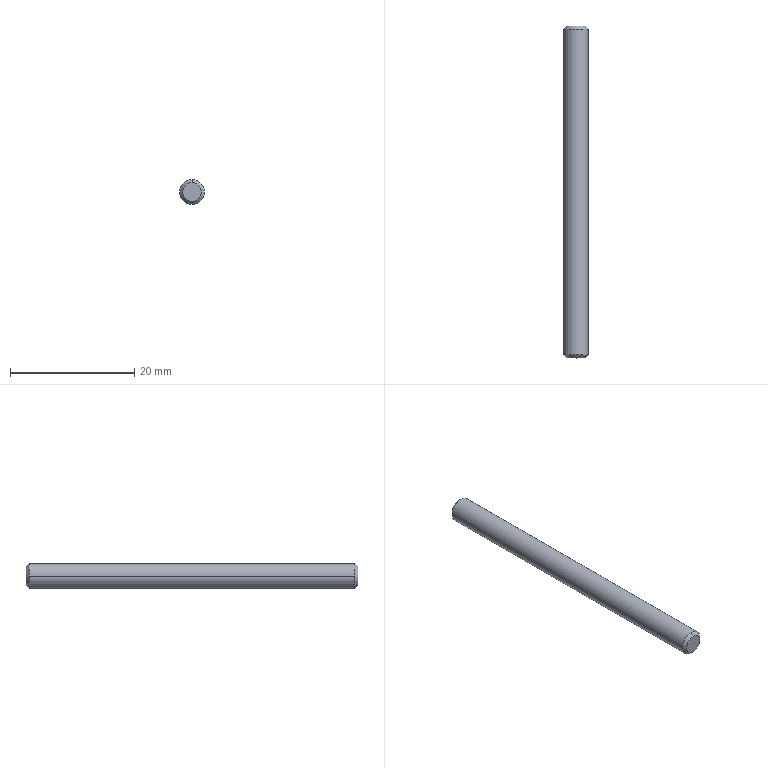Part | STEP file | 1 solid | 8 faces | box 4 x 53.4 x 4 mm | volume 668.164 mm3 | cone 4 | cylinder 2 | plane 2 | commonest cylinder face diameters 4 x2
STEP:
#1=CARTESIAN_POINT('',(0.,0.,0.));
#2=DIRECTION('',(0.,0.,1.));
#3=DIRECTION('',(1.,0.,0.));
#4=AXIS2_PLACEMENT_3D('',#1,#2,#3);
#5=CARTESIAN_POINT('',(0.,-26.7,-1.5));
#6=VERTEX_POINT('',#5);
#7=CARTESIAN_POINT('',(0.,-26.7,1.5));
#8=VERTEX_POINT('',#7);
#9=CARTESIAN_POINT('',(0.,-26.7,0.));
#10=DIRECTION('',(0.,-1.,0.));
#11=DIRECTION('',(0.,0.,1.));
#12=AXIS2_PLACEMENT_3D('',#9,#10,#11);
#13=CIRCLE('',#12,1.5);
#14=CARTESIAN_POINT('',(0.,-26.7,0.));
#15=DIRECTION('',(0.,1.,0.));
#16=DIRECTION('',(0.,0.,1.));
#17=AXIS2_PLACEMENT_3D('',#14,#15,#16);
#18=CONICAL_SURFACE('',#17,1.5,0.7854);
#19=CARTESIAN_POINT('',(6.283,0.));
#20=DIRECTION('',(-1.,0.));
#21=VECTOR('',#20,1.);
#22=LINE('',#19,#21);
#23=(GEOMETRIC_REPRESENTATION_CONTEXT(2)PARAMETRIC_REPRESENTATION_CONTEXT()REPRESENTATION_CONTEXT('',''));
#24=DEFINITIONAL_REPRESENTATION('',(#22),#23);
#25=PCURVE('',#18,#24);
#26=CARTESIAN_POINT('',(-1.518,-26.7,-1.518));
#27=DIRECTION('',(0.,1.,0.));
#28=DIRECTION('',(0.,0.,1.));
#29=AXIS2_PLACEMENT_3D('',#26,#27,#28);
#30=PLANE('',#29);
#31=CARTESIAN_POINT('',(3.018,1.518));
#32=CARTESIAN_POINT('',(3.018,-1.08));
#33=CARTESIAN_POINT('',(0.768,0.219));
#34=CARTESIAN_POINT('',(-1.482,1.518));
#35=CARTESIAN_POINT('',(0.768,2.817));
#36=CARTESIAN_POINT('',(3.018,4.116));
#37=CARTESIAN_POINT('',(3.018,1.518));
#38=(BOUNDED_CURVE()B_SPLINE_CURVE(2,(#31,#32,#33,#34,#35,#36,#37),.UNSPECIFIED.,.T.,.F.)B_SPLINE_CURVE_WITH_KNOTS((1,2,2,2,2,1),(-2.094,0.,2.094,4.189,6.283,8.378),.UNSPECIFIED.)CURVE()GEOMETRIC_REPRESENTATION_ITEM()RATIONAL_B_SPLINE_CURVE((1.,0.5,1.,0.5,1.,0.5,1.))REPRESENTATION_ITEM(''));
#39=(GEOMETRIC_REPRESENTATION_CONTEXT(2)PARAMETRIC_REPRESENTATION_CONTEXT()REPRESENTATION_CONTEXT('',''));
#40=DEFINITIONAL_REPRESENTATION('',(#38),#39);
#41=PCURVE('',#30,#40);
#42=SURFACE_CURVE('',#13,(#25,#41),.PCURVE_S1.);
#43=EDGE_CURVE('',#6,#8,#42,.T.);
#44=ORIENTED_EDGE('',*,*,#43,.F.);
#45=CARTESIAN_POINT('',(0.,-26.2,-2.));
#46=VERTEX_POINT('',#45);
#47=CARTESIAN_POINT('',(0.,-26.7,-1.5));
#48=DIRECTION('',(0.,0.7071,-0.7071));
#49=VECTOR('',#48,1.);
#50=LINE('',#47,#49);
#51=CARTESIAN_POINT('',(3.142,0.));
#52=DIRECTION('',(0.,1.));
#53=VECTOR('',#52,1.);
#54=LINE('',#51,#53);
#55=(GEOMETRIC_REPRESENTATION_CONTEXT(2)PARAMETRIC_REPRESENTATION_CONTEXT()REPRESENTATION_CONTEXT('',''));
#56=DEFINITIONAL_REPRESENTATION('',(#54),#55);
#57=PCURVE('',#18,#56);
#58=CARTESIAN_POINT('',(0.,-26.7,0.));
#59=DIRECTION('',(0.,1.,0.));
#60=DIRECTION('',(0.,0.,1.));
#61=AXIS2_PLACEMENT_3D('',#58,#59,#60);
#62=CONICAL_SURFACE('',#61,1.5,0.7854);
#63=CARTESIAN_POINT('',(3.142,0.));
#64=DIRECTION('',(0.,1.));
#65=VECTOR('',#64,1.);
#66=LINE('',#63,#65);
#67=(GEOMETRIC_REPRESENTATION_CONTEXT(2)PARAMETRIC_REPRESENTATION_CONTEXT()REPRESENTATION_CONTEXT('',''));
#68=DEFINITIONAL_REPRESENTATION('',(#66),#67);
#69=PCURVE('',#62,#68);
#70=SURFACE_CURVE('',#50,(#57,#69),.PCURVE_S1.);
#71=EDGE_CURVE('',#6,#46,#70,.T.);
#72=ORIENTED_EDGE('',*,*,#71,.T.);
#73=CARTESIAN_POINT('',(2.,-26.2,0.));
#74=VERTEX_POINT('',#73);
#75=CARTESIAN_POINT('',(0.,-26.2,0.));
#76=DIRECTION('',(0.,1.,0.));
#77=DIRECTION('',(0.,0.,1.));
#78=AXIS2_PLACEMENT_3D('',#75,#76,#77);
#79=CIRCLE('',#78,2.);
#80=CARTESIAN_POINT('',(0.,0.5));
#81=DIRECTION('',(1.,0.));
#82=VECTOR('',#81,1.);
#83=LINE('',#80,#82);
#84=(GEOMETRIC_REPRESENTATION_CONTEXT(2)PARAMETRIC_REPRESENTATION_CONTEXT()REPRESENTATION_CONTEXT('',''));
#85=DEFINITIONAL_REPRESENTATION('',(#83),#84);
#86=PCURVE('',#18,#85);
#87=CARTESIAN_POINT('',(0.,-26.2,0.));
#88=DIRECTION('',(0.,1.,0.));
#89=DIRECTION('',(-1.,0.,0.));
#90=AXIS2_PLACEMENT_3D('',#87,#88,#89);
#91=CYLINDRICAL_SURFACE('',#90,2.);
#92=CARTESIAN_POINT('',(1.571,0.));
#93=DIRECTION('',(1.,0.));
#94=VECTOR('',#93,1.);
#95=LINE('',#92,#94);
#96=(GEOMETRIC_REPRESENTATION_CONTEXT(2)PARAMETRIC_REPRESENTATION_CONTEXT()REPRESENTATION_CONTEXT('',''));
#97=DEFINITIONAL_REPRESENTATION('',(#95),#96);
#98=PCURVE('',#91,#97);
#99=SURFACE_CURVE('',#79,(#86,#98),.PCURVE_S1.);
#100=EDGE_CURVE('',#74,#46,#99,.T.);
#101=ORIENTED_EDGE('',*,*,#100,.F.);
#102=CARTESIAN_POINT('',(0.,-26.2,2.));
#103=VERTEX_POINT('',#102);
#104=CARTESIAN_POINT('',(0.,-26.2,0.));
#105=DIRECTION('',(0.,1.,0.));
#106=DIRECTION('',(0.,0.,1.));
#107=AXIS2_PLACEMENT_3D('',#104,#105,#106);
#108=CIRCLE('',#107,2.);
#109=CARTESIAN_POINT('',(0.,0.5));
#110=DIRECTION('',(1.,0.));
#111=VECTOR('',#110,1.);
#112=LINE('',#109,#111);
#113=(GEOMETRIC_REPRESENTATION_CONTEXT(2)PARAMETRIC_REPRESENTATION_CONTEXT()REPRESENTATION_CONTEXT('',''));
#114=DEFINITIONAL_REPRESENTATION('',(#112),#113);
#115=PCURVE('',#18,#114);
#116=CARTESIAN_POINT('',(0.,-26.2,0.));
#117=DIRECTION('',(0.,1.,0.));
#118=DIRECTION('',(-1.,0.,0.));
#119=AXIS2_PLACEMENT_3D('',#116,#117,#118);
#120=CYLINDRICAL_SURFACE('',#119,2.);
#121=CARTESIAN_POINT('',(1.571,0.));
#122=DIRECTION('',(1.,0.));
#123=VECTOR('',#122,1.);
#124=LINE('',#121,#123);
#125=(GEOMETRIC_REPRESENTATION_CONTEXT(2)PARAMETRIC_REPRESENTATION_CONTEXT()REPRESENTATION_CONTEXT('',''));
#126=DEFINITIONAL_REPRESENTATION('',(#124),#125);
#127=PCURVE('',#120,#126);
#128=SURFACE_CURVE('',#108,(#115,#127),.PCURVE_S1.);
#129=EDGE_CURVE('',#103,#74,#128,.T.);
#130=ORIENTED_EDGE('',*,*,#129,.F.);
#131=CARTESIAN_POINT('',(0.,-26.7,1.5));
#132=DIRECTION('',(0.,0.7071,0.7071));
#133=VECTOR('',#132,1.);
#134=LINE('',#131,#133);
#135=CARTESIAN_POINT('',(0.,0.));
#136=DIRECTION('',(0.,1.));
#137=VECTOR('',#136,1.);
#138=LINE('',#135,#137);
#139=(GEOMETRIC_REPRESENTATION_CONTEXT(2)PARAMETRIC_REPRESENTATION_CONTEXT()REPRESENTATION_CONTEXT('',''));
#140=DEFINITIONAL_REPRESENTATION('',(#138),#139);
#141=PCURVE('',#18,#140);
#142=CARTESIAN_POINT('',(6.283,0.));
#143=DIRECTION('',(0.,1.));
#144=VECTOR('',#143,1.);
#145=LINE('',#142,#144);
#146=(GEOMETRIC_REPRESENTATION_CONTEXT(2)PARAMETRIC_REPRESENTATION_CONTEXT()REPRESENTATION_CONTEXT('',''));
#147=DEFINITIONAL_REPRESENTATION('',(#145),#146);
#148=PCURVE('',#62,#147);
#149=SURFACE_CURVE('',#134,(#141,#148),.PCURVE_S1.);
#150=EDGE_CURVE('',#8,#103,#149,.T.);
#151=ORIENTED_EDGE('',*,*,#150,.F.);
#152=EDGE_LOOP('',(#44,#72,#101,#130,#151));
#153=FACE_BOUND('',#152,.T.);
#154=ADVANCED_FACE('',(#153),#18,.T.);
#155=CARTESIAN_POINT('',(-2.,-26.2,0.));
#156=VERTEX_POINT('',#155);
#157=CARTESIAN_POINT('',(0.,-26.2,0.));
#158=DIRECTION('',(0.,1.,0.));
#159=DIRECTION('',(0.,0.,1.));
#160=AXIS2_PLACEMENT_3D('',#157,#158,#159);
#161=CIRCLE('',#160,2.);
#162=CARTESIAN_POINT('',(-4.712,0.));
#163=DIRECTION('',(1.,0.));
#164=VECTOR('',#163,1.);
#165=LINE('',#162,#164);
#166=(GEOMETRIC_REPRESENTATION_CONTEXT(2)PARAMETRIC_REPRESENTATION_CONTEXT()REPRESENTATION_CONTEXT('',''));
#167=DEFINITIONAL_REPRESENTATION('',(#165),#166);
#168=PCURVE('',#120,#167);
#169=CARTESIAN_POINT('',(0.,0.5));
#170=DIRECTION('',(1.,0.));
#171=VECTOR('',#170,1.);
#172=LINE('',#169,#171);
#173=(GEOMETRIC_REPRESENTATION_CONTEXT(2)PARAMETRIC_REPRESENTATION_CONTEXT()REPRESENTATION_CONTEXT('',''));
#174=DEFINITIONAL_REPRESENTATION('',(#172),#173);
#175=PCURVE('',#62,#174);
#176=SURFACE_CURVE('',#161,(#168,#175),.PCURVE_S1.);
#177=EDGE_CURVE('',#156,#103,#176,.T.);
#178=ORIENTED_EDGE('',*,*,#177,.T.);
#179=ORIENTED_EDGE('',*,*,#129,.T.);
#180=CARTESIAN_POINT('',(2.,26.2,0.));
#181=VERTEX_POINT('',#180);
#182=CARTESIAN_POINT('',(2.,-26.2,0.));
#183=DIRECTION('',(0.,1.,0.));
#184=VECTOR('',#183,1.);
#185=LINE('',#182,#184);
#186=CARTESIAN_POINT('',(3.142,0.));
#187=DIRECTION('',(0.,1.));
#188=VECTOR('',#187,1.);
#189=LINE('',#186,#188);
#190=(GEOMETRIC_REPRESENTATION_CONTEXT(2)PARAMETRIC_REPRESENTATION_CONTEXT()REPRESENTATION_CONTEXT('',''));
#191=DEFINITIONAL_REPRESENTATION('',(#189),#190);
#192=PCURVE('',#120,#191);
#193=CARTESIAN_POINT('',(3.142,0.));
#194=DIRECTION('',(0.,1.));
#195=VECTOR('',#194,1.);
#196=LINE('',#193,#195);
#197=(GEOMETRIC_REPRESENTATION_CONTEXT(2)PARAMETRIC_REPRESENTATION_CONTEXT()REPRESENTATION_CONTEXT('',''));
#198=DEFINITIONAL_REPRESENTATION('',(#196),#197);
#199=PCURVE('',#91,#198);
#200=SURFACE_CURVE('',#185,(#192,#199),.PCURVE_S1.);
#201=EDGE_CURVE('',#74,#181,#200,.T.);
#202=ORIENTED_EDGE('',*,*,#201,.T.);
#203=CARTESIAN_POINT('',(0.,26.2,2.));
#204=VERTEX_POINT('',#203);
#205=CARTESIAN_POINT('',(0.,26.2,0.));
#206=DIRECTION('',(0.,1.,0.));
#207=DIRECTION('',(0.,0.,1.));
#208=AXIS2_PLACEMENT_3D('',#205,#206,#207);
#209=CIRCLE('',#208,2.);
#210=CARTESIAN_POINT('',(1.571,52.4));
#211=DIRECTION('',(1.,0.));
#212=VECTOR('',#211,1.);
#213=LINE('',#210,#212);
#214=(GEOMETRIC_REPRESENTATION_CONTEXT(2)PARAMETRIC_REPRESENTATION_CONTEXT()REPRESENTATION_CONTEXT('',''));
#215=DEFINITIONAL_REPRESENTATION('',(#213),#214);
#216=PCURVE('',#120,#215);
#217=CARTESIAN_POINT('',(0.,26.7,0.));
#218=DIRECTION('',(0.,-1.,0.));
#219=DIRECTION('',(0.,0.,-1.));
#220=AXIS2_PLACEMENT_3D('',#217,#218,#219);
#221=CONICAL_SURFACE('',#220,1.5,0.7854);
#222=CARTESIAN_POINT('',(3.142,0.5));
#223=DIRECTION('',(-1.,0.));
#224=VECTOR('',#223,1.);
#225=LINE('',#222,#224);
#226=(GEOMETRIC_REPRESENTATION_CONTEXT(2)PARAMETRIC_REPRESENTATION_CONTEXT()REPRESENTATION_CONTEXT('',''));
#227=DEFINITIONAL_REPRESENTATION('',(#225),#226);
#228=PCURVE('',#221,#227);
#229=SURFACE_CURVE('',#209,(#216,#228),.PCURVE_S1.);
#230=EDGE_CURVE('',#204,#181,#229,.T.);
#231=ORIENTED_EDGE('',*,*,#230,.F.);
#232=CARTESIAN_POINT('',(-2.,26.2,0.));
#233=VERTEX_POINT('',#232);
#234=CARTESIAN_POINT('',(0.,26.2,0.));
#235=DIRECTION('',(0.,1.,0.));
#236=DIRECTION('',(0.,0.,1.));
#237=AXIS2_PLACEMENT_3D('',#234,#235,#236);
#238=CIRCLE('',#237,2.);
#239=CARTESIAN_POINT('',(-4.712,52.4));
#240=DIRECTION('',(1.,0.));
#241=VECTOR('',#240,1.);
#242=LINE('',#239,#241);
#243=(GEOMETRIC_REPRESENTATION_CONTEXT(2)PARAMETRIC_REPRESENTATION_CONTEXT()REPRESENTATION_CONTEXT('',''));
#244=DEFINITIONAL_REPRESENTATION('',(#242),#243);
#245=PCURVE('',#120,#244);
#246=CARTESIAN_POINT('',(0.,26.7,0.));
#247=DIRECTION('',(0.,-1.,0.));
#248=DIRECTION('',(0.,0.,-1.));
#249=AXIS2_PLACEMENT_3D('',#246,#247,#248);
#250=CONICAL_SURFACE('',#249,1.5,0.7854);
#251=CARTESIAN_POINT('',(9.425,0.5));
#252=DIRECTION('',(-1.,0.));
#253=VECTOR('',#252,1.);
#254=LINE('',#251,#253);
#255=(GEOMETRIC_REPRESENTATION_CONTEXT(2)PARAMETRIC_REPRESENTATION_CONTEXT()REPRESENTATION_CONTEXT('',''));
#256=DEFINITIONAL_REPRESENTATION('',(#254),#255);
#257=PCURVE('',#250,#256);
#258=SURFACE_CURVE('',#238,(#245,#257),.PCURVE_S1.);
#259=EDGE_CURVE('',#233,#204,#258,.T.);
#260=ORIENTED_EDGE('',*,*,#259,.F.);
#261=CARTESIAN_POINT('',(-2.,-26.2,0.));
#262=DIRECTION('',(0.,1.,0.));
#263=VECTOR('',#262,1.);
#264=LINE('',#261,#263);
#265=CARTESIAN_POINT('',(0.,0.));
#266=DIRECTION('',(0.,1.));
#267=VECTOR('',#266,1.);
#268=LINE('',#265,#267);
#269=(GEOMETRIC_REPRESENTATION_CONTEXT(2)PARAMETRIC_REPRESENTATION_CONTEXT()REPRESENTATION_CONTEXT('',''));
#270=DEFINITIONAL_REPRESENTATION('',(#268),#269);
#271=PCURVE('',#120,#270);
#272=CARTESIAN_POINT('',(6.283,0.));
#273=DIRECTION('',(0.,1.));
#274=VECTOR('',#273,1.);
#275=LINE('',#272,#274);
#276=(GEOMETRIC_REPRESENTATION_CONTEXT(2)PARAMETRIC_REPRESENTATION_CONTEXT()REPRESENTATION_CONTEXT('',''));
#277=DEFINITIONAL_REPRESENTATION('',(#275),#276);
#278=PCURVE('',#91,#277);
#279=SURFACE_CURVE('',#264,(#271,#278),.PCURVE_S1.);
#280=EDGE_CURVE('',#156,#233,#279,.T.);
#281=ORIENTED_EDGE('',*,*,#280,.F.);
#282=EDGE_LOOP('',(#178,#179,#202,#231,#260,#281));
#283=FACE_BOUND('',#282,.T.);
#284=ADVANCED_FACE('',(#283),#120,.T.);
#285=CARTESIAN_POINT('',(0.,26.7,1.5));
#286=VERTEX_POINT('',#285);
#287=CARTESIAN_POINT('',(0.,26.7,-1.5));
#288=VERTEX_POINT('',#287);
#289=CARTESIAN_POINT('',(0.,26.7,0.));
#290=DIRECTION('',(0.,1.,0.));
#291=DIRECTION('',(0.,0.,-1.));
#292=AXIS2_PLACEMENT_3D('',#289,#290,#291);
#293=CIRCLE('',#292,1.5);
#294=CARTESIAN_POINT('',(6.283,0.));
#295=DIRECTION('',(-1.,0.));
#296=VECTOR('',#295,1.);
#297=LINE('',#294,#296);
#298=(GEOMETRIC_REPRESENTATION_CONTEXT(2)PARAMETRIC_REPRESENTATION_CONTEXT()REPRESENTATION_CONTEXT('',''));
#299=DEFINITIONAL_REPRESENTATION('',(#297),#298);
#300=PCURVE('',#221,#299);
#301=CARTESIAN_POINT('',(-1.518,26.7,1.518));
#302=DIRECTION('',(0.,-1.,0.));
#303=DIRECTION('',(0.,0.,-1.));
#304=AXIS2_PLACEMENT_3D('',#301,#302,#303);
#305=PLANE('',#304);
#306=CARTESIAN_POINT('',(3.018,1.518));
#307=CARTESIAN_POINT('',(3.018,-1.08));
#308=CARTESIAN_POINT('',(0.768,0.219));
#309=CARTESIAN_POINT('',(-1.482,1.518));
#310=CARTESIAN_POINT('',(0.768,2.817));
#311=CARTESIAN_POINT('',(3.018,4.116));
#312=CARTESIAN_POINT('',(3.018,1.518));
#313=(BOUNDED_CURVE()B_SPLINE_CURVE(2,(#306,#307,#308,#309,#310,#311,#312),.UNSPECIFIED.,.T.,.F.)B_SPLINE_CURVE_WITH_KNOTS((1,2,2,2,2,1),(-2.094,0.,2.094,4.189,6.283,8.378),.UNSPECIFIED.)CURVE()GEOMETRIC_REPRESENTATION_ITEM()RATIONAL_B_SPLINE_CURVE((1.,0.5,1.,0.5,1.,0.5,1.))REPRESENTATION_ITEM(''));
#314=(GEOMETRIC_REPRESENTATION_CONTEXT(2)PARAMETRIC_REPRESENTATION_CONTEXT()REPRESENTATION_CONTEXT('',''));
#315=DEFINITIONAL_REPRESENTATION('',(#313),#314);
#316=PCURVE('',#305,#315);
#317=SURFACE_CURVE('',#293,(#300,#316),.PCURVE_S1.);
#318=EDGE_CURVE('',#286,#288,#317,.T.);
#319=ORIENTED_EDGE('',*,*,#318,.F.);
#320=CARTESIAN_POINT('',(0.,26.7,1.5));
#321=DIRECTION('',(0.,-0.7071,0.7071));
#322=VECTOR('',#321,1.);
#323=LINE('',#320,#322);
#324=CARTESIAN_POINT('',(3.142,0.));
#325=DIRECTION('',(0.,1.));
#326=VECTOR('',#325,1.);
#327=LINE('',#324,#326);
#328=(GEOMETRIC_REPRESENTATION_CONTEXT(2)PARAMETRIC_REPRESENTATION_CONTEXT()REPRESENTATION_CONTEXT('',''));
#329=DEFINITIONAL_REPRESENTATION('',(#327),#328);
#330=PCURVE('',#221,#329);
#331=CARTESIAN_POINT('',(3.142,0.));
#332=DIRECTION('',(0.,1.));
#333=VECTOR('',#332,1.);
#334=LINE('',#331,#333);
#335=(GEOMETRIC_REPRESENTATION_CONTEXT(2)PARAMETRIC_REPRESENTATION_CONTEXT()REPRESENTATION_CONTEXT('',''));
#336=DEFINITIONAL_REPRESENTATION('',(#334),#335);
#337=PCURVE('',#250,#336);
#338=SURFACE_CURVE('',#323,(#330,#337),.PCURVE_S1.);
#339=EDGE_CURVE('',#286,#204,#338,.T.);
#340=ORIENTED_EDGE('',*,*,#339,.T.);
#341=ORIENTED_EDGE('',*,*,#230,.T.);
#342=CARTESIAN_POINT('',(0.,26.2,-2.));
#343=VERTEX_POINT('',#342);
#344=CARTESIAN_POINT('',(0.,26.2,0.));
#345=DIRECTION('',(0.,1.,0.));
#346=DIRECTION('',(0.,0.,1.));
#347=AXIS2_PLACEMENT_3D('',#344,#345,#346);
#348=CIRCLE('',#347,2.);
#349=CARTESIAN_POINT('',(3.142,0.5));
#350=DIRECTION('',(-1.,0.));
#351=VECTOR('',#350,1.);
#352=LINE('',#349,#351);
#353=(GEOMETRIC_REPRESENTATION_CONTEXT(2)PARAMETRIC_REPRESENTATION_CONTEXT()REPRESENTATION_CONTEXT('',''));
#354=DEFINITIONAL_REPRESENTATION('',(#352),#353);
#355=PCURVE('',#221,#354);
#356=CARTESIAN_POINT('',(1.571,52.4));
#357=DIRECTION('',(1.,0.));
#358=VECTOR('',#357,1.);
#359=LINE('',#356,#358);
#360=(GEOMETRIC_REPRESENTATION_CONTEXT(2)PARAMETRIC_REPRESENTATION_CONTEXT()REPRESENTATION_CONTEXT('',''));
#361=DEFINITIONAL_REPRESENTATION('',(#359),#360);
#362=PCURVE('',#91,#361);
#363=SURFACE_CURVE('',#348,(#355,#362),.PCURVE_S1.);
#364=EDGE_CURVE('',#181,#343,#363,.T.);
#365=ORIENTED_EDGE('',*,*,#364,.T.);
#366=CARTESIAN_POINT('',(0.,26.7,-1.5));
#367=DIRECTION('',(0.,-0.7071,-0.7071));
#368=VECTOR('',#367,1.);
#369=LINE('',#366,#368);
#370=CARTESIAN_POINT('',(0.,0.));
#371=DIRECTION('',(0.,1.));
#372=VECTOR('',#371,1.);
#373=LINE('',#370,#372);
#374=(GEOMETRIC_REPRESENTATION_CONTEXT(2)PARAMETRIC_REPRESENTATION_CONTEXT()REPRESENTATION_CONTEXT('',''));
#375=DEFINITIONAL_REPRESENTATION('',(#373),#374);
#376=PCURVE('',#221,#375);
#377=CARTESIAN_POINT('',(6.283,0.));
#378=DIRECTION('',(0.,1.));
#379=VECTOR('',#378,1.);
#380=LINE('',#377,#379);
#381=(GEOMETRIC_REPRESENTATION_CONTEXT(2)PARAMETRIC_REPRESENTATION_CONTEXT()REPRESENTATION_CONTEXT('',''));
#382=DEFINITIONAL_REPRESENTATION('',(#380),#381);
#383=PCURVE('',#250,#382);
#384=SURFACE_CURVE('',#369,(#376,#383),.PCURVE_S1.);
#385=EDGE_CURVE('',#288,#343,#384,.T.);
#386=ORIENTED_EDGE('',*,*,#385,.F.);
#387=EDGE_LOOP('',(#319,#340,#341,#365,#386));
#388=FACE_BOUND('',#387,.T.);
#389=ADVANCED_FACE('',(#388),#221,.T.);
#390=ORIENTED_EDGE('',*,*,#71,.F.);
#391=CARTESIAN_POINT('',(0.,-26.7,0.));
#392=DIRECTION('',(0.,-1.,0.));
#393=DIRECTION('',(0.,0.,1.));
#394=AXIS2_PLACEMENT_3D('',#391,#392,#393);
#395=CIRCLE('',#394,1.5);
#396=CARTESIAN_POINT('',(6.283,0.));
#397=DIRECTION('',(-1.,0.));
#398=VECTOR('',#397,1.);
#399=LINE('',#396,#398);
#400=(GEOMETRIC_REPRESENTATION_CONTEXT(2)PARAMETRIC_REPRESENTATION_CONTEXT()REPRESENTATION_CONTEXT('',''));
#401=DEFINITIONAL_REPRESENTATION('',(#399),#400);
#402=PCURVE('',#62,#401);
#403=CARTESIAN_POINT('',(3.018,1.518));
#404=CARTESIAN_POINT('',(3.018,-1.08));
#405=CARTESIAN_POINT('',(0.768,0.219));
#406=CARTESIAN_POINT('',(-1.482,1.518));
#407=CARTESIAN_POINT('',(0.768,2.817));
#408=CARTESIAN_POINT('',(3.018,4.116));
#409=CARTESIAN_POINT('',(3.018,1.518));
#410=(BOUNDED_CURVE()B_SPLINE_CURVE(2,(#403,#404,#405,#406,#407,#408,#409),.UNSPECIFIED.,.T.,.F.)B_SPLINE_CURVE_WITH_KNOTS((1,2,2,2,2,1),(-2.094,0.,2.094,4.189,6.283,8.378),.UNSPECIFIED.)CURVE()GEOMETRIC_REPRESENTATION_ITEM()RATIONAL_B_SPLINE_CURVE((1.,0.5,1.,0.5,1.,0.5,1.))REPRESENTATION_ITEM(''));
#411=(GEOMETRIC_REPRESENTATION_CONTEXT(2)PARAMETRIC_REPRESENTATION_CONTEXT()REPRESENTATION_CONTEXT('',''));
#412=DEFINITIONAL_REPRESENTATION('',(#410),#411);
#413=PCURVE('',#30,#412);
#414=SURFACE_CURVE('',#395,(#402,#413),.PCURVE_S1.);
#415=EDGE_CURVE('',#8,#6,#414,.T.);
#416=ORIENTED_EDGE('',*,*,#415,.F.);
#417=ORIENTED_EDGE('',*,*,#150,.T.);
#418=ORIENTED_EDGE('',*,*,#177,.F.);
#419=CARTESIAN_POINT('',(0.,-26.2,0.));
#420=DIRECTION('',(0.,1.,0.));
#421=DIRECTION('',(0.,0.,1.));
#422=AXIS2_PLACEMENT_3D('',#419,#420,#421);
#423=CIRCLE('',#422,2.);
#424=CARTESIAN_POINT('',(0.,0.5));
#425=DIRECTION('',(1.,0.));
#426=VECTOR('',#425,1.);
#427=LINE('',#424,#426);
#428=(GEOMETRIC_REPRESENTATION_CONTEXT(2)PARAMETRIC_REPRESENTATION_CONTEXT()REPRESENTATION_CONTEXT('',''));
#429=DEFINITIONAL_REPRESENTATION('',(#427),#428);
#430=PCURVE('',#62,#429);
#431=CARTESIAN_POINT('',(1.571,0.));
#432=DIRECTION('',(1.,0.));
#433=VECTOR('',#432,1.);
#434=LINE('',#431,#433);
#435=(GEOMETRIC_REPRESENTATION_CONTEXT(2)PARAMETRIC_REPRESENTATION_CONTEXT()REPRESENTATION_CONTEXT('',''));
#436=DEFINITIONAL_REPRESENTATION('',(#434),#435);
#437=PCURVE('',#91,#436);
#438=SURFACE_CURVE('',#423,(#430,#437),.PCURVE_S1.);
#439=EDGE_CURVE('',#46,#156,#438,.T.);
#440=ORIENTED_EDGE('',*,*,#439,.F.);
#441=EDGE_LOOP('',(#390,#416,#417,#418,#440));
#442=FACE_BOUND('',#441,.T.);
#443=ADVANCED_FACE('',(#442),#62,.T.);
#444=ORIENTED_EDGE('',*,*,#415,.T.);
#445=ORIENTED_EDGE('',*,*,#43,.T.);
#446=EDGE_LOOP('',(#444,#445));
#447=FACE_BOUND('',#446,.T.);
#448=ADVANCED_FACE('',(#447),#30,.F.);
#449=ORIENTED_EDGE('',*,*,#201,.F.);
#450=ORIENTED_EDGE('',*,*,#100,.T.);
#451=ORIENTED_EDGE('',*,*,#439,.T.);
#452=ORIENTED_EDGE('',*,*,#280,.T.);
#453=CARTESIAN_POINT('',(0.,26.2,0.));
#454=DIRECTION('',(0.,1.,0.));
#455=DIRECTION('',(0.,0.,1.));
#456=AXIS2_PLACEMENT_3D('',#453,#454,#455);
#457=CIRCLE('',#456,2.);
#458=CARTESIAN_POINT('',(1.571,52.4));
#459=DIRECTION('',(1.,0.));
#460=VECTOR('',#459,1.);
#461=LINE('',#458,#460);
#462=(GEOMETRIC_REPRESENTATION_CONTEXT(2)PARAMETRIC_REPRESENTATION_CONTEXT()REPRESENTATION_CONTEXT('',''));
#463=DEFINITIONAL_REPRESENTATION('',(#461),#462);
#464=PCURVE('',#91,#463);
#465=CARTESIAN_POINT('',(9.425,0.5));
#466=DIRECTION('',(-1.,0.));
#467=VECTOR('',#466,1.);
#468=LINE('',#465,#467);
#469=(GEOMETRIC_REPRESENTATION_CONTEXT(2)PARAMETRIC_REPRESENTATION_CONTEXT()REPRESENTATION_CONTEXT('',''));
#470=DEFINITIONAL_REPRESENTATION('',(#468),#469);
#471=PCURVE('',#250,#470);
#472=SURFACE_CURVE('',#457,(#464,#471),.PCURVE_S1.);
#473=EDGE_CURVE('',#343,#233,#472,.T.);
#474=ORIENTED_EDGE('',*,*,#473,.F.);
#475=ORIENTED_EDGE('',*,*,#364,.F.);
#476=EDGE_LOOP('',(#449,#450,#451,#452,#474,#475));
#477=FACE_BOUND('',#476,.T.);
#478=ADVANCED_FACE('',(#477),#91,.T.);
#479=ORIENTED_EDGE('',*,*,#339,.F.);
#480=CARTESIAN_POINT('',(0.,26.7,0.));
#481=DIRECTION('',(0.,1.,0.));
#482=DIRECTION('',(0.,0.,-1.));
#483=AXIS2_PLACEMENT_3D('',#480,#481,#482);
#484=CIRCLE('',#483,1.5);
#485=CARTESIAN_POINT('',(6.283,0.));
#486=DIRECTION('',(-1.,0.));
#487=VECTOR('',#486,1.);
#488=LINE('',#485,#487);
#489=(GEOMETRIC_REPRESENTATION_CONTEXT(2)PARAMETRIC_REPRESENTATION_CONTEXT()REPRESENTATION_CONTEXT('',''));
#490=DEFINITIONAL_REPRESENTATION('',(#488),#489);
#491=PCURVE('',#250,#490);
#492=CARTESIAN_POINT('',(3.018,1.518));
#493=CARTESIAN_POINT('',(3.018,-1.08));
#494=CARTESIAN_POINT('',(0.768,0.219));
#495=CARTESIAN_POINT('',(-1.482,1.518));
#496=CARTESIAN_POINT('',(0.768,2.817));
#497=CARTESIAN_POINT('',(3.018,4.116));
#498=CARTESIAN_POINT('',(3.018,1.518));
#499=(BOUNDED_CURVE()B_SPLINE_CURVE(2,(#492,#493,#494,#495,#496,#497,#498),.UNSPECIFIED.,.T.,.F.)B_SPLINE_CURVE_WITH_KNOTS((1,2,2,2,2,1),(-2.094,0.,2.094,4.189,6.283,8.378),.UNSPECIFIED.)CURVE()GEOMETRIC_REPRESENTATION_ITEM()RATIONAL_B_SPLINE_CURVE((1.,0.5,1.,0.5,1.,0.5,1.))REPRESENTATION_ITEM(''));
#500=(GEOMETRIC_REPRESENTATION_CONTEXT(2)PARAMETRIC_REPRESENTATION_CONTEXT()REPRESENTATION_CONTEXT('',''));
#501=DEFINITIONAL_REPRESENTATION('',(#499),#500);
#502=PCURVE('',#305,#501);
#503=SURFACE_CURVE('',#484,(#491,#502),.PCURVE_S1.);
#504=EDGE_CURVE('',#288,#286,#503,.T.);
#505=ORIENTED_EDGE('',*,*,#504,.F.);
#506=ORIENTED_EDGE('',*,*,#385,.T.);
#507=ORIENTED_EDGE('',*,*,#473,.T.);
#508=ORIENTED_EDGE('',*,*,#259,.T.);
#509=EDGE_LOOP('',(#479,#505,#506,#507,#508));
#510=FACE_BOUND('',#509,.T.);
#511=ADVANCED_FACE('',(#510),#250,.T.);
#512=ORIENTED_EDGE('',*,*,#504,.T.);
#513=ORIENTED_EDGE('',*,*,#318,.T.);
#514=EDGE_LOOP('',(#512,#513));
#515=FACE_BOUND('',#514,.T.);
#516=ADVANCED_FACE('',(#515),#305,.F.);
#517=CLOSED_SHELL('',(#154,#284,#389,#443,#448,#478,#511,#516));
#518=MANIFOLD_SOLID_BREP('',#517);
#519=(LENGTH_UNIT()NAMED_UNIT(*)SI_UNIT(.MILLI.,.METRE.));
#520=UNCERTAINTY_MEASURE_WITH_UNIT(LENGTH_MEASURE(0.0000001),#519,'','');
#521=(NAMED_UNIT(*)PLANE_ANGLE_UNIT()SI_UNIT($,.RADIAN.));
#522=(NAMED_UNIT(*)SI_UNIT($,.STERADIAN.)SOLID_ANGLE_UNIT());
#523=(GEOMETRIC_REPRESENTATION_CONTEXT(3)GLOBAL_UNCERTAINTY_ASSIGNED_CONTEXT((#520))GLOBAL_UNIT_ASSIGNED_CONTEXT((#519,#521,#522))REPRESENTATION_CONTEXT('',''));
#524=ADVANCED_BREP_SHAPE_REPRESENTATION('',(#4,#518),#523);